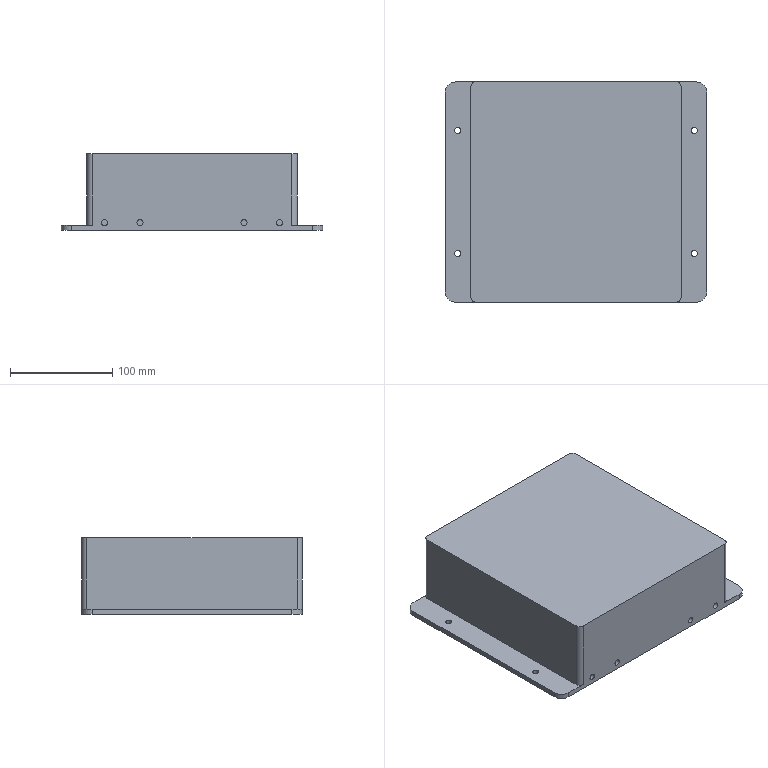NC program | NX | posted with a generic post | part box 255 x 215 x 75 mm
Lines 119 to 1998 of 11258:
(FLOOR_WALL_1_COPY_1 , TOOL : D16)
N224 T18 M6
N226 G54
N228 G17 G0 G90 X-0.676 Y-8. B0. C0. S9500 M3
N230 G43 Z30. H18
N232 Z1.5
N234 G94 G1 X3. Z1.307 F1000.
N236 Y8. Z0.469
N238 X-3. Z0.154
N240 Y-8. Z-0.684
N242 X3. Z-0.999
N244 Y8. F2500.
N246 X-3.
N248 Y-8.
N250 X3.
N252 Y-17.6
N254 X12.6
N256 Y17.6
N258 X-12.6
N260 Y-17.6
N262 X3.
N264 Y-27.2
N266 X22.2
N268 Y27.2
N270 X-22.2
N272 Y-27.2
N274 X3.
N276 Y-36.8
N278 X31.8
N280 Y36.8
N282 X-31.8
N284 Y-36.8
N286 X3.
N288 Y-46.4
N290 X41.4
N292 Y46.4
N294 X-41.4
N296 Y-46.4
N298 X3.
N300 Y-56.
N302 X51.
N304 Y56.
N306 X-51.
N308 Y-56.
N310 X3.
N312 Y-65.6
N314 X60.6
N316 Y65.6
N318 X-60.6
N320 Y-65.6
N322 X3.
N324 Y-75.2
N326 X70.2
N328 Y75.2
N330 X-70.2
N332 Y-75.2
N334 X3.
N336 Y-84.8
N338 X79.8
N340 Y84.8
N342 X-79.8
N344 Y-84.8
N346 X3.
N348 Y-94.4
N350 X89.4
N352 Y94.4
N354 X-89.4
N356 Y-94.4
N358 X3.
N360 Z0.501
N362 G0 X-0.676 Y-8.
N364 G1 X3. Z0.309 F1000.
N366 Y8. Z-0.53
N368 X-3. Z-0.844
N370 Y-8. Z-1.683
N372 X3. Z-1.997
N374 Y8. F2500.
N376 X-3.
N378 Y-8.
N380 X3.
N382 Y-17.6
N384 X12.6
N386 Y17.6
N388 X-12.6
N390 Y-17.6
N392 X3.
N394 Y-27.2
N396 X22.2
N398 Y27.2
N400 X-22.2
N402 Y-27.2
N404 X3.
N406 Y-36.8
N408 X31.8
N410 Y36.8
N412 X-31.8
N414 Y-36.8
N416 X3.
N418 Y-46.4
N420 X41.4
N422 Y46.4
N424 X-41.4
N426 Y-46.4
N428 X3.
N430 Y-56.
N432 X51.
N434 Y56.
N436 X-51.
N438 Y-56.
N440 X3.
N442 Y-65.6
N444 X60.6
N446 Y65.6
N448 X-60.6
N450 Y-65.6
N452 X3.
N454 Y-75.2
N456 X70.2
N458 Y75.2
N460 X-70.2
N462 Y-75.2
N464 X3.
N466 Y-84.8
N468 X79.8
N470 Y84.8
N472 X-79.8
N474 Y-84.8
N476 X3.
N478 Y-94.4
N480 X89.4
N482 Y94.4
N484 X-89.4
N486 Y-94.4
N488 X3.
N490 Z-0.497
N492 G0 X-0.676 Y-8.
N494 G1 X3. Z-0.69 F1000.
N496 Y8. Z-1.528
N498 X-3. Z-1.843
N500 Y-8. Z-2.681
N502 X3. Z-2.996
N504 Y8. F2500.
N506 X-3.
N508 Y-8.
N510 X3.
N512 Y-17.6
N514 X12.6
N516 Y17.6
N518 X-12.6
N520 Y-17.6
N522 X3.
N524 Y-27.2
N526 X22.2
N528 Y27.2
N530 X-22.2
N532 Y-27.2
N534 X3.
N536 Y-36.8
N538 X31.8
N540 Y36.8
N542 X-31.8
N544 Y-36.8
N546 X3.
N548 Y-46.4
N550 X41.4
N552 Y46.4
N554 X-41.4
N556 Y-46.4
N558 X3.
N560 Y-56.
N562 X51.
N564 Y56.
N566 X-51.
N568 Y-56.
N570 X3.
N572 Y-65.6
N574 X60.6
N576 Y65.6
N578 X-60.6
N580 Y-65.6
N582 X3.
N584 Y-75.2
N586 X70.2
N588 Y75.2
N590 X-70.2
N592 Y-75.2
N594 X3.
N596 Y-84.8
N598 X79.8
N600 Y84.8
N602 X-79.8
N604 Y-84.8
N606 X3.
N608 Y-94.4
N610 X89.4
N612 Y94.4
N614 X-89.4
N616 Y-94.4
N618 X3.
N620 Z-1.496
N622 G0 X-0.676 Y-8.
N624 G1 X3. Z-1.688 F1000.
N626 Y8. Z-2.527
N628 X-3. Z-2.841
N630 Y-8. Z-3.68
N632 X3. Z-3.994
N634 Y8. F2500.
N636 X-3.
N638 Y-8.
N640 X3.
N642 Y-17.6
N644 X12.6
N646 Y17.6
N648 X-12.6
N650 Y-17.6
N652 X3.
N654 Y-27.2
N656 X22.2
N658 Y27.2
N660 X-22.2
N662 Y-27.2
N664 X3.
N666 Y-36.8
N668 X31.8
N670 Y36.8
N672 X-31.8
N674 Y-36.8
N676 X3.
N678 Y-46.4
N680 X41.4
N682 Y46.4
N684 X-41.4
N686 Y-46.4
N688 X3.
N690 Y-56.
N692 X51.
N694 Y56.
N696 X-51.
N698 Y-56.
N700 X3.
N702 Y-65.6
N704 X60.6
N706 Y65.6
N708 X-60.6
N710 Y-65.6
N712 X3.
N714 Y-75.2
N716 X70.2
N718 Y75.2
N720 X-70.2
N722 Y-75.2
N724 X3.
N726 Y-84.8
N728 X79.8
N730 Y84.8
N732 X-79.8
N734 Y-84.8
N736 X3.
N738 Y-94.4
N740 X89.4
N742 Y94.4
N744 X-89.4
N746 Y-94.4
N748 X3.
N750 Z-2.494
N752 G0 X-0.676 Y-8.
N754 G1 X3. Z-2.687 F1000.
N756 Y8. Z-3.525
N758 X-3. Z-3.84
N760 Y-8. Z-4.678
N762 X3. Z-4.993
N764 Y8. F2500.
N766 X-3.
N768 Y-8.
N770 X3.
N772 Y-17.6
N774 X12.6
N776 Y17.6
N778 X-12.6
N780 Y-17.6
N782 X3.
N784 Y-27.2
N786 X22.2
N788 Y27.2
N790 X-22.2
N792 Y-27.2
N794 X3.
N796 Y-36.8
N798 X31.8
N800 Y36.8
N802 X-31.8
N804 Y-36.8
N806 X3.
N808 Y-46.4
N810 X41.4
N812 Y46.4
N814 X-41.4
N816 Y-46.4
N818 X3.
N820 Y-56.
N822 X51.
N824 Y56.
N826 X-51.
N828 Y-56.
N830 X3.
N832 Y-65.6
N834 X60.6
N836 Y65.6
N838 X-60.6
N840 Y-65.6
N842 X3.
N844 Y-75.2
N846 X70.2
N848 Y75.2
N850 X-70.2
N852 Y-75.2
N854 X3.
N856 Y-84.8
N858 X79.8
N860 Y84.8
N862 X-79.8
N864 Y-84.8
N866 X3.
N868 Y-94.4
N870 X89.4
N872 Y94.4
N874 X-89.4
N876 Y-94.4
N878 X3.
N880 Z-3.493
N882 G0 X-0.676 Y-8.
N884 G1 X3. Z-3.685 F1000.
N886 Y8. Z-4.524
N888 X-3. Z-4.838
N890 Y-8. Z-5.677
N892 X3. Z-5.991
N894 Y8. F2500.
N896 X-3.
N898 Y-8.
N900 X3.
N902 Y-17.6
N904 X12.6
N906 Y17.6
N908 X-12.6
N910 Y-17.6
N912 X3.
N914 Y-27.2
N916 X22.2
N918 Y27.2
N920 X-22.2
N922 Y-27.2
N924 X3.
N926 Y-36.8
N928 X31.8
N930 Y36.8
N932 X-31.8
N934 Y-36.8
N936 X3.
N938 Y-46.4
N940 X41.4
N942 Y46.4
N944 X-41.4
N946 Y-46.4
N948 X3.
N950 Y-56.
N952 X51.
N954 Y56.
N956 X-51.
N958 Y-56.
N960 X3.
N962 Y-65.6
N964 X60.6
N966 Y65.6
N968 X-60.6
N970 Y-65.6
N972 X3.
N974 Y-75.2
N976 X70.2
N978 Y75.2
N980 X-70.2
N982 Y-75.2
N984 X3.
N986 Y-84.8
N988 X79.8
N990 Y84.8
N992 X-79.8
N994 Y-84.8
N996 X3.
N998 Y-94.4
N1000 X89.4
N1002 Y94.4
N1004 X-89.4
N1006 Y-94.4
N1008 X3.
N1010 Z-4.491
N1012 G0 X-0.676 Y-8.
N1014 G1 X3. Z-4.684 F1000.
N1016 Y8. Z-5.523
N1018 X-3. Z-5.837
N1020 Y-8. Z-6.676
N1022 X3. Z-6.99
N1024 Y8. F2500.
N1026 X-3.
N1028 Y-8.
N1030 X3.
N1032 Y-17.6
N1034 X12.6
N1036 Y17.6
N1038 X-12.6
N1040 Y-17.6
N1042 X3.
N1044 Y-27.2
N1046 X22.2
N1048 Y27.2
N1050 X-22.2
N1052 Y-27.2
N1054 X3.
N1056 Y-36.8
N1058 X31.8
N1060 Y36.8
N1062 X-31.8
N1064 Y-36.8
N1066 X3.
N1068 Y-46.4
N1070 X41.4
N1072 Y46.4
N1074 X-41.4
N1076 Y-46.4
N1078 X3.
N1080 Y-56.
N1082 X51.
N1084 Y56.
N1086 X-51.
N1088 Y-56.
N1090 X3.
N1092 Y-65.6
N1094 X60.6
N1096 Y65.6
N1098 X-60.6
N1100 Y-65.6
N1102 X3.
N1104 Y-75.2
N1106 X70.2
N1108 Y75.2
N1110 X-70.2
N1112 Y-75.2
N1114 X3.
N1116 Y-84.8
N1118 X79.8
N1120 Y84.8
N1122 X-79.8
N1124 Y-84.8
N1126 X3.
N1128 Y-94.4
N1130 X89.4
N1132 Y94.4
N1134 X-89.4
N1136 Y-94.4
N1138 X3.
N1140 Z-5.49
N1142 G0 X-0.676 Y-8.
N1144 G1 X3. Z-5.683 F1000.
N1146 Y8. Z-6.521
N1148 X-3. Z-6.836
N1150 Y-8. Z-7.674
N1152 X3. Z-7.989
N1154 Y8. F2500.
N1156 X-3.
N1158 Y-8.
N1160 X3.
N1162 Y-17.6
N1164 X12.6
N1166 Y17.6
N1168 X-12.6
N1170 Y-17.6
N1172 X3.
N1174 Y-27.2
N1176 X22.2
N1178 Y27.2
N1180 X-22.2
N1182 Y-27.2
N1184 X3.
N1186 Y-36.8
N1188 X31.8
N1190 Y36.8
N1192 X-31.8
N1194 Y-36.8
N1196 X3.
N1198 Y-46.4
N1200 X41.4
N1202 Y46.4
N1204 X-41.4
N1206 Y-46.4
N1208 X3.
N1210 Y-56.
N1212 X51.
N1214 Y56.
N1216 X-51.
N1218 Y-56.
N1220 X3.
N1222 Y-65.6
N1224 X60.6
N1226 Y65.6
N1228 X-60.6
N1230 Y-65.6
N1232 X3.
N1234 Y-75.2
N1236 X70.2
N1238 Y75.2
N1240 X-70.2
N1242 Y-75.2
N1244 X3.
N1246 Y-84.8
N1248 X79.8
N1250 Y84.8
N1252 X-79.8
N1254 Y-84.8
N1256 X3.
N1258 Y-94.4
N1260 X89.4
N1262 Y94.4
N1264 X-89.4
N1266 Y-94.4
N1268 X3.
N1270 Z-6.489
N1272 G0 X-0.676 Y-8.
N1274 G1 X3. Z-6.681 F1000.
N1276 Y8. Z-7.52
N1278 X-3. Z-7.834
N1280 Y-8. Z-8.673
N1282 X3. Z-8.987
N1284 Y8. F2500.
N1286 X-3.
N1288 Y-8.
N1290 X3.
N1292 Y-17.6
N1294 X12.6
N1296 Y17.6
N1298 X-12.6
N1300 Y-17.6
N1302 X3.
N1304 Y-27.2
N1306 X22.2
N1308 Y27.2
N1310 X-22.2
N1312 Y-27.2
N1314 X3.
N1316 Y-36.8
N1318 X31.8
N1320 Y36.8
N1322 X-31.8
N1324 Y-36.8
N1326 X3.
N1328 Y-46.4
N1330 X41.4
N1332 Y46.4
N1334 X-41.4
N1336 Y-46.4
N1338 X3.
N1340 Y-56.
N1342 X51.
N1344 Y56.
N1346 X-51.
N1348 Y-56.
N1350 X3.
N1352 Y-65.6
N1354 X60.6
N1356 Y65.6
N1358 X-60.6
N1360 Y-65.6
N1362 X3.
N1364 Y-75.2
N1366 X70.2
N1368 Y75.2
N1370 X-70.2
N1372 Y-75.2
N1374 X3.
N1376 Y-84.8
N1378 X79.8
N1380 Y84.8
N1382 X-79.8
N1384 Y-84.8
N1386 X3.
N1388 Y-94.4
N1390 X89.4
N1392 Y94.4
N1394 X-89.4
N1396 Y-94.4
N1398 X3.
N1400 Z-7.487
N1402 G0 X-0.676 Y-8.
N1404 G1 X3. Z-7.68 F1000.
N1406 Y8. Z-8.518
N1408 X-3. Z-8.833
N1410 Y-8. Z-9.671
N1412 X3. Z-9.986
N1414 Y8. F2500.
N1416 X-3.
N1418 Y-8.
N1420 X3.
N1422 Y-17.6
N1424 X12.6
N1426 Y17.6
N1428 X-12.6
N1430 Y-17.6
N1432 X3.
N1434 Y-27.2
N1436 X22.2
N1438 Y27.2
N1440 X-22.2
N1442 Y-27.2
N1444 X3.
N1446 Y-36.8
N1448 X31.8
N1450 Y36.8
N1452 X-31.8
N1454 Y-36.8
N1456 X3.
N1458 Y-46.4
N1460 X41.4
N1462 Y46.4
N1464 X-41.4
N1466 Y-46.4
N1468 X3.
N1470 Y-56.
N1472 X51.
N1474 Y56.
N1476 X-51.
N1478 Y-56.
N1480 X3.
N1482 Y-65.6
N1484 X60.6
N1486 Y65.6
N1488 X-60.6
N1490 Y-65.6
N1492 X3.
N1494 Y-75.2
N1496 X70.2
N1498 Y75.2
N1500 X-70.2
N1502 Y-75.2
N1504 X3.
N1506 Y-84.8
N1508 X79.8
N1510 Y84.8
N1512 X-79.8
N1514 Y-84.8
N1516 X3.
N1518 Y-94.4
N1520 X89.4
N1522 Y94.4
N1524 X-89.4
N1526 Y-94.4
N1528 X3.
N1530 Z-8.486
N1532 G0 X-0.676 Y-8.
N1534 G1 X3. Z-8.678 F1000.
N1536 Y8. Z-9.517
N1538 X-3. Z-9.831
N1540 Y-8. Z-10.67
N1542 X3. Z-10.984
N1544 Y8. F2500.
N1546 X-3.
N1548 Y-8.
N1550 X3.
N1552 Y-17.6
N1554 X12.6
N1556 Y17.6
N1558 X-12.6
N1560 Y-17.6
N1562 X3.
N1564 Y-27.2
N1566 X22.2
N1568 Y27.2
N1570 X-22.2
N1572 Y-27.2
N1574 X3.
N1576 Y-36.8
N1578 X31.8
N1580 Y36.8
N1582 X-31.8
N1584 Y-36.8
N1586 X3.
N1588 Y-46.4
N1590 X41.4
N1592 Y46.4
N1594 X-41.4
N1596 Y-46.4
N1598 X3.
N1600 Y-56.
N1602 X51.
N1604 Y56.
N1606 X-51.
N1608 Y-56.
N1610 X3.
N1612 Y-65.6
N1614 X60.6
N1616 Y65.6
N1618 X-60.6
N1620 Y-65.6
N1622 X3.
N1624 Y-75.2
N1626 X70.2
N1628 Y75.2
N1630 X-70.2
N1632 Y-75.2
N1634 X3.
N1636 Y-84.8
N1638 X79.8
N1640 Y84.8
N1642 X-79.8
N1644 Y-84.8
N1646 X3.
N1648 Y-94.4
N1650 X89.4
N1652 Y94.4
N1654 X-89.4
N1656 Y-94.4
N1658 X3.
N1660 Z-9.484
N1662 G0 X-0.676 Y-8.
N1664 G1 X3. Z-9.677 F1000.
N1666 Y8. Z-10.515
N1668 X-3. Z-10.83
N1670 Y-8. Z-11.668
N1672 X3. Z-11.983
N1674 Y8. F2500.
N1676 X-3.
N1678 Y-8.
N1680 X3.
N1682 Y-17.6
N1684 X12.6
N1686 Y17.6
N1688 X-12.6
N1690 Y-17.6
N1692 X3.
N1694 Y-27.2
N1696 X22.2
N1698 Y27.2
N1700 X-22.2
N1702 Y-27.2
N1704 X3.
N1706 Y-36.8
N1708 X31.8
N1710 Y36.8
N1712 X-31.8
N1714 Y-36.8
N1716 X3.
N1718 Y-46.4
N1720 X41.4
N1722 Y46.4
N1724 X-41.4
N1726 Y-46.4
N1728 X3.
N1730 Y-56.
N1732 X51.
N1734 Y56.
N1736 X-51.
N1738 Y-56.
N1740 X3.
N1742 Y-65.6
N1744 X60.6
N1746 Y65.6
N1748 X-60.6
N1750 Y-65.6
N1752 X3.
N1754 Y-75.2
N1756 X70.2
N1758 Y75.2
N1760 X-70.2
N1762 Y-75.2
N1764 X3.
N1766 Y-84.8
N1768 X79.8
N1770 Y84.8
N1772 X-79.8
N1774 Y-84.8
N1776 X3.
N1778 Y-94.4
N1780 X89.4
N1782 Y94.4
N1784 X-89.4
N1786 Y-94.4
N1788 X3.
N1790 Z-10.483
N1792 G0 X-0.676 Y-8.
N1794 G1 X3. Z-10.675 F1000.
N1796 Y8. Z-11.514
N1798 X-3. Z-11.828
N1800 Y-8. Z-12.667
N1802 X3. Z-12.981
N1804 Y8. F2500.
N1806 X-3.
N1808 Y-8.
N1810 X3.
N1812 Y-17.6
N1814 X12.6
N1816 Y17.6
N1818 X-12.6
N1820 Y-17.6
N1822 X3.
N1824 Y-27.2
N1826 X22.2
N1828 Y27.2
N1830 X-22.2
N1832 Y-27.2
N1834 X3.
N1836 Y-36.8
N1838 X31.8
N1840 Y36.8
N1842 X-31.8
N1844 Y-36.8
N1846 X3.
N1848 Y-46.4
N1850 X41.4
N1852 Y46.4
N1854 X-41.4
N1856 Y-46.4
N1858 X3.
N1860 Y-56.
N1862 X51.
N1864 Y56.
N1866 X-51.
N1868 Y-56.
N1870 X3.
N1872 Y-65.6
N1874 X60.6
N1876 Y65.6
N1878 X-60.6
N1880 Y-65.6
N1882 X3.
N1884 Y-75.2
N1886 X70.2
N1888 Y75.2
N1890 X-70.2
N1892 Y-75.2
N1894 X3.
N1896 Y-84.8
N1898 X79.8
N1900 Y84.8
N1902 X-79.8
N1904 Y-84.8
N1906 X3.
N1908 Y-94.4
N1910 X89.4
N1912 Y94.4
N1914 X-89.4
N1916 Y-94.4
N1918 X3.
N1920 Z-11.481
N1922 G0 X-0.676 Y-8.
N1924 G1 X3. Z-11.674 F1000.
N1926 Y8. Z-12.513
N1928 X-3. Z-12.827
N1930 Y-8. Z-13.666
N1932 X3. Z-13.98
N1934 Y8. F2500.
N1936 X-3.
N1938 Y-8.
N1940 X3.
N1942 Y-17.6
N1944 X12.6
N1946 Y17.6
N1948 X-12.6
N1950 Y-17.6
N1952 X3.
N1954 Y-27.2
N1956 X22.2
N1958 Y27.2
N1960 X-22.2
N1962 Y-27.2
N1964 X3.
N1966 Y-36.8
N1968 X31.8
N1970 Y36.8
N1972 X-31.8
N1974 Y-36.8
N1976 X3.
N1978 Y-46.4
N1980 X41.4
N1982 Y46.4
N1984 X-41.4
N1986 Y-46.4
N1988 X3.
N1990 Y-56.
N1992 X51.
N1994 Y56.
N1996 X-51.
N1998 Y-56.
N2000 X3.
N2002 Y-65.6
N2004 X60.6
N2006 Y65.6
N2008 X-60.6
N2010 Y-65.6
N2012 X3.
N2014 Y-75.2
N2016 X70.2
N2018 Y75.2
N2020 X-70.2
N2022 Y-75.2
N2024 X3.
N2026 Y-84.8
N2028 X79.8
N2030 Y84.8
N2032 X-79.8
N2034 Y-84.8
N2036 X3.
N2038 Y-94.4
N2040 X89.4
N2042 Y94.4
N2044 X-89.4
N2046 Y-94.4
N2048 X3.
N2050 Z-12.48
N2052 G0 X-0.676 Y-8.
N2054 G1 X3. Z-12.673 F1000.
N2056 Y8. Z-13.511
N2058 X-3. Z-13.826
N2060 Y-8. Z-14.664
N2062 X3. Z-14.979
N2064 Y8. F2500.
N2066 X-3.
N2068 Y-8.
N2070 X3.
N2072 Y-17.6
N2074 X12.6
N2076 Y17.6
N2078 X-12.6
N2080 Y-17.6
N2082 X3.
N2084 Y-27.2
N2086 X22.2
N2088 Y27.2
N2090 X-22.2
N2092 Y-27.2
N2094 X3.
N2096 Y-36.8
N2098 X31.8
N2100 Y36.8
N2102 X-31.8
N2104 Y-36.8
N2106 X3.
N2108 Y-46.4
N2110 X41.4
N2112 Y46.4
N2114 X-41.4
N2116 Y-46.4
N2118 X3.
N2120 Y-56.
N2122 X51.
N2124 Y56.
N2126 X-51.
N2128 Y-56.
N2130 X3.
N2132 Y-65.6
N2134 X60.6
N2136 Y65.6
N2138 X-60.6
N2140 Y-65.6
N2142 X3.
N2144 Y-75.2
N2146 X70.2
N2148 Y75.2
N2150 X-70.2
N2152 Y-75.2
N2154 X3.
N2156 Y-84.8
N2158 X79.8
N2160 Y84.8
N2162 X-79.8
N2164 Y-84.8
N2166 X3.
N2168 Y-94.4
N2170 X89.4
N2172 Y94.4
N2174 X-89.4
N2176 Y-94.4
N2178 X3.
N2180 Z-13.479
N2182 G0 X-0.676 Y-8.
N2184 G1 X3. Z-13.671 F1000.
N2186 Y8. Z-14.51
N2188 X-3. Z-14.824
N2190 Y-8. Z-15.663
N2192 X3. Z-15.977
N2194 Y8. F2500.
N2196 X-3.
N2198 Y-8.
N2200 X3.
N2202 Y-17.6
N2204 X12.6
N2206 Y17.6
N2208 X-12.6
N2210 Y-17.6
N2212 X3.
N2214 Y-27.2
N2216 X22.2
N2218 Y27.2
N2220 X-22.2
N2222 Y-27.2
N2224 X3.
N2226 Y-36.8
N2228 X31.8
N2230 Y36.8
N2232 X-31.8
N2234 Y-36.8
N2236 X3.
N2238 Y-46.4
N2240 X41.4
N2242 Y46.4
N2244 X-41.4
N2246 Y-46.4
N2248 X3.
N2250 Y-56.
N2252 X51.
N2254 Y56.
N2256 X-51.
N2258 Y-56.
N2260 X3.
N2262 Y-65.6
N2264 X60.6
N2266 Y65.6
N2268 X-60.6
N2270 Y-65.6
N2272 X3.
N2274 Y-75.2
N2276 X70.2
N2278 Y75.2
N2280 X-70.2
N2282 Y-75.2
N2284 X3.
N2286 Y-84.8
N2288 X79.8
N2290 Y84.8
N2292 X-79.8
N2294 Y-84.8
N2296 X3.
N2298 Y-94.4
N2300 X89.4
N2302 Y94.4
N2304 X-89.4
N2306 Y-94.4
N2308 X3.
N2310 Z-14.477
N2312 G0 X-0.676 Y-8.
N2314 G1 X3. Z-14.67 F1000.
N2316 Y8. Z-15.508
N2318 X-3. Z-15.823
N2320 Y-8. Z-16.661
N2322 X3. Z-16.976
N2324 Y8. F2500.
N2326 X-3.
N2328 Y-8.
N2330 X3.
N2332 Y-17.6
N2334 X12.6
N2336 Y17.6
N2338 X-12.6
N2340 Y-17.6
N2342 X3.
N2344 Y-27.2
N2346 X22.2
N2348 Y27.2
N2350 X-22.2
N2352 Y-27.2
N2354 X3.
N2356 Y-36.8
N2358 X31.8
N2360 Y36.8
N2362 X-31.8
N2364 Y-36.8
N2366 X3.
N2368 Y-46.4
N2370 X41.4
N2372 Y46.4
N2374 X-41.4
N2376 Y-46.4
N2378 X3.
N2380 Y-56.
N2382 X51.
N2384 Y56.
N2386 X-51.
N2388 Y-56.
N2390 X3.
N2392 Y-65.6
N2394 X60.6
N2396 Y65.6
N2398 X-60.6
N2400 Y-65.6
N2402 X3.
N2404 Y-75.2
N2406 X70.2
N2408 Y75.2
N2410 X-70.2
N2412 Y-75.2
N2414 X3.
N2416 Y-84.8
N2418 X79.8
N2420 Y84.8
N2422 X-79.8
N2424 Y-84.8
N2426 X3.
N2428 Y-94.4
N2430 X89.4
N2432 Y94.4
N2434 X-89.4
N2436 Y-94.4
N2438 X3.
N2440 Z-15.476
N2442 G0 X-0.676 Y-8.
N2444 G1 X3. Z-15.668 F1000.
N2446 Y8. Z-16.507
N2448 X-3. Z-16.821
N2450 Y-8. Z-17.66
N2452 X3. Z-17.974
N2454 Y8. F2500.
N2456 X-3.
N2458 Y-8.
N2460 X3.
N2462 Y-17.6
N2464 X12.6
N2466 Y17.6
N2468 X-12.6
N2470 Y-17.6
N2472 X3.
N2474 Y-27.2
N2476 X22.2
N2478 Y27.2
N2480 X-22.2
N2482 Y-27.2
N2484 X3.
N2486 Y-36.8
N2488 X31.8
N2490 Y36.8
N2492 X-31.8
N2494 Y-36.8
N2496 X3.
N2498 Y-46.4
N2500 X41.4
N2502 Y46.4
N2504 X-41.4
N2506 Y-46.4
N2508 X3.
N2510 Y-56.
N2512 X51.
N2514 Y56.
N2516 X-51.
N2518 Y-56.
N2520 X3.
N2522 Y-65.6
N2524 X60.6
N2526 Y65.6
N2528 X-60.6
N2530 Y-65.6
N2532 X3.
N2534 Y-75.2
N2536 X70.2
N2538 Y75.2
N2540 X-70.2
N2542 Y-75.2
N2544 X3.
N2546 Y-84.8
N2548 X79.8
N2550 Y84.8
N2552 X-79.8
N2554 Y-84.8
N2556 X3.
N2558 Y-94.4
N2560 X89.4
N2562 Y94.4
N2564 X-89.4
N2566 Y-94.4
N2568 X3.
N2570 Z-16.474
N2572 G0 X-0.676 Y-8.
N2574 G1 X3. Z-16.667 F1000.
N2576 Y8. Z-17.505
N2578 X-3. Z-17.82
N2580 Y-8. Z-18.658
N2582 X3. Z-18.973
N2584 Y8. F2500.
N2586 X-3.
N2588 Y-8.
N2590 X3.
N2592 Y-17.6
N2594 X12.6
N2596 Y17.6
N2598 X-12.6
N2600 Y-17.6
N2602 X3.
N2604 Y-27.2
N2606 X22.2
N2608 Y27.2
N2610 X-22.2
N2612 Y-27.2
N2614 X3.
N2616 Y-36.8
N2618 X31.8
N2620 Y36.8
N2622 X-31.8
N2624 Y-36.8
N2626 X3.
N2628 Y-46.4
N2630 X41.4
N2632 Y46.4
N2634 X-41.4
N2636 Y-46.4
N2638 X3.
N2640 Y-56.
N2642 X51.
N2644 Y56.
N2646 X-51.
N2648 Y-56.
N2650 X3.
N2652 Y-65.6
N2654 X60.6
N2656 Y65.6
N2658 X-60.6
N2660 Y-65.6
N2662 X3.
N2664 Y-75.2
N2666 X70.2
N2668 Y75.2
N2670 X-70.2
N2672 Y-75.2
N2674 X3.
N2676 Y-84.8
N2678 X79.8
N2680 Y84.8
N2682 X-79.8
N2684 Y-84.8
N2686 X3.
N2688 Y-94.4
N2690 X89.4
N2692 Y94.4
N2694 X-89.4
N2696 Y-94.4
N2698 X3.
N2700 Z-17.473
N2702 G0 X-0.676 Y-8.
N2704 G1 X3. Z-17.665 F1000.
N2706 Y8. Z-18.504
N2708 X-3. Z-18.818
N2710 Y-8. Z-19.657
N2712 X3. Z-19.971
N2714 Y8. F2500.
N2716 X-3.
N2718 Y-8.
N2720 X3.
N2722 Y-17.6
N2724 X12.6
N2726 Y17.6
N2728 X-12.6
N2730 Y-17.6
N2732 X3.
N2734 Y-27.2
N2736 X22.2
N2738 Y27.2
N2740 X-22.2
N2742 Y-27.2
N2744 X3.
N2746 Y-36.8
N2748 X31.8
N2750 Y36.8
N2752 X-31.8
N2754 Y-36.8
N2756 X3.
N2758 Y-46.4
N2760 X41.4
N2762 Y46.4
N2764 X-41.4
N2766 Y-46.4
N2768 X3.
N2770 Y-56.
N2772 X51.
N2774 Y56.
N2776 X-51.
N2778 Y-56.
N2780 X3.
N2782 Y-65.6
N2784 X60.6
N2786 Y65.6
N2788 X-60.6
N2790 Y-65.6
N2792 X3.
N2794 Y-75.2
N2796 X70.2
N2798 Y75.2
N2800 X-70.2
N2802 Y-75.2
N2804 X3.
N2806 Y-84.8
N2808 X79.8
N2810 Y84.8
N2812 X-79.8
N2814 Y-84.8
N2816 X3.
N2818 Y-94.4
N2820 X89.4
N2822 Y94.4
N2824 X-89.4
N2826 Y-94.4
N2828 X3.
N2830 Z-18.471
N2832 G0 X-0.676 Y-8.
N2834 G1 X3. Z-18.664 F1000.
N2836 Y8. Z-19.503
N2838 X-3. Z-19.817
N2840 Y-8. Z-20.656
N2842 X3. Z-20.97
N2844 Y8. F2500.
N2846 X-3.
N2848 Y-8.
N2850 X3.
N2852 Y-17.6
N2854 X12.6
N2856 Y17.6
N2858 X-12.6
N2860 Y-17.6
N2862 X3.
N2864 Y-27.2
N2866 X22.2
N2868 Y27.2
N2870 X-22.2
N2872 Y-27.2
N2874 X3.
N2876 Y-36.8
N2878 X31.8
N2880 Y36.8
N2882 X-31.8
N2884 Y-36.8
N2886 X3.
N2888 Y-46.4
N2890 X41.4
N2892 Y46.4
N2894 X-41.4
N2896 Y-46.4
N2898 X3.
N2900 Y-56.
N2902 X51.
N2904 Y56.
N2906 X-51.
N2908 Y-56.
N2910 X3.
N2912 Y-65.6
N2914 X60.6
N2916 Y65.6
N2918 X-60.6
N2920 Y-65.6
N2922 X3.
N2924 Y-75.2
N2926 X70.2
N2928 Y75.2
N2930 X-70.2
N2932 Y-75.2
N2934 X3.
N2936 Y-84.8
N2938 X79.8
N2940 Y84.8
N2942 X-79.8
N2944 Y-84.8
N2946 X3.
N2948 Y-94.4
N2950 X89.4
N2952 Y94.4
N2954 X-89.4
N2956 Y-94.4
N2958 X3.
N2960 Z-19.47
N2962 G0 X-0.676 Y-8.
N2964 G1 X3. Z-19.663 F1000.
N2966 Y8. Z-20.501
N2968 X-3. Z-20.816
N2970 Y-8. Z-21.654
N2972 X3. Z-21.969
N2974 Y8. F2500.
N2976 X-3.
N2978 Y-8.
N2980 X3.
N2982 Y-17.6
N2984 X12.6
N2986 Y17.6
N2988 X-12.6
N2990 Y-17.6
N2992 X3.
N2994 Y-27.2
N2996 X22.2
N2998 Y27.2
N3000 X-22.2
N3002 Y-27.2
N3004 X3.
N3006 Y-36.8
N3008 X31.8
N3010 Y36.8
N3012 X-31.8
N3014 Y-36.8
N3016 X3.
N3018 Y-46.4
N3020 X41.4
N3022 Y46.4
N3024 X-41.4
N3026 Y-46.4
N3028 X3.
N3030 Y-56.
N3032 X51.
N3034 Y56.
N3036 X-51.
N3038 Y-56.
N3040 X3.
N3042 Y-65.6
N3044 X60.6
N3046 Y65.6
N3048 X-60.6
N3050 Y-65.6
N3052 X3.
N3054 Y-75.2
N3056 X70.2
N3058 Y75.2
N3060 X-70.2
N3062 Y-75.2
N3064 X3.
N3066 Y-84.8
N3068 X79.8
N3070 Y84.8
N3072 X-79.8
N3074 Y-84.8
N3076 X3.
N3078 Y-94.4
N3080 X89.4
N3082 Y94.4
N3084 X-89.4
N3086 Y-94.4
N3088 X3.
N3090 Z-20.469
N3092 G0 X-0.676 Y-8.
N3094 G1 X3. Z-20.661 F1000.
N3096 Y8. Z-21.5
N3098 X-3. Z-21.814
N3100 Y-8. Z-22.653
N3102 X3. Z-22.967
N3104 Y8. F2500.
N3106 X-3.
N3108 Y-8.
N3110 X3.
N3112 Y-17.6
N3114 X12.6
N3116 Y17.6
N3118 X-12.6
N3120 Y-17.6
N3122 X3.
N3124 Y-27.2
N3126 X22.2
N3128 Y27.2
N3130 X-22.2
N3132 Y-27.2
N3134 X3.
N3136 Y-36.8
N3138 X31.8
N3140 Y36.8
N3142 X-31.8
N3144 Y-36.8
N3146 X3.
N3148 Y-46.4
N3150 X41.4
N3152 Y46.4
N3154 X-41.4
N3156 Y-46.4
N3158 X3.
N3160 Y-56.
N3162 X51.
N3164 Y56.
N3166 X-51.
N3168 Y-56.
N3170 X3.
N3172 Y-65.6
N3174 X60.6
N3176 Y65.6
N3178 X-60.6
N3180 Y-65.6
N3182 X3.
N3184 Y-75.2
N3186 X70.2
N3188 Y75.2
N3190 X-70.2
N3192 Y-75.2
N3194 X3.
N3196 Y-84.8
N3198 X79.8
N3200 Y84.8
N3202 X-79.8
N3204 Y-84.8
N3206 X3.
N3208 Y-94.4
N3210 X89.4
N3212 Y94.4
N3214 X-89.4
N3216 Y-94.4
N3218 X3.
N3220 Z-21.467
N3222 G0 X-0.676 Y-8.
N3224 G1 X3. Z-21.66 F1000.
N3226 Y8. Z-22.498
N3228 X-3. Z-22.813
N3230 Y-8. Z-23.651
N3232 X3. Z-23.966
N3234 Y8. F2500.
N3236 X-3.
N3238 Y-8.
N3240 X3.
N3242 Y-17.6
N3244 X12.6
N3246 Y17.6
N3248 X-12.6
N3250 Y-17.6
N3252 X3.
N3254 Y-27.2
N3256 X22.2
N3258 Y27.2
N3260 X-22.2
N3262 Y-27.2
N3264 X3.
N3266 Y-36.8
N3268 X31.8
N3270 Y36.8
N3272 X-31.8
N3274 Y-36.8
N3276 X3.
N3278 Y-46.4
N3280 X41.4
N3282 Y46.4
N3284 X-41.4
N3286 Y-46.4
N3288 X3.
N3290 Y-56.
N3292 X51.
N3294 Y56.
N3296 X-51.
N3298 Y-56.
N3300 X3.
N3302 Y-65.6
N3304 X60.6
N3306 Y65.6
N3308 X-60.6
N3310 Y-65.6
N3312 X3.
N3314 Y-75.2
N3316 X70.2
N3318 Y75.2
N3320 X-70.2
N3322 Y-75.2
N3324 X3.
N3326 Y-84.8
N3328 X79.8
N3330 Y84.8
N3332 X-79.8
N3334 Y-84.8
N3336 X3.
N3338 Y-94.4
N3340 X89.4
N3342 Y94.4
N3344 X-89.4
N3346 Y-94.4
N3348 X3.
N3350 Z-22.466
N3352 G0 X-0.676 Y-8.
N3354 G1 X3. Z-22.658 F1000.
N3356 Y8. Z-23.497
N3358 X-3. Z-23.811
N3360 Y-8. Z-24.65
N3362 X3. Z-24.964
N3364 Y8. F2500.
N3366 X-3.
N3368 Y-8.
N3370 X3.
N3372 Y-17.6
N3374 X12.6
N3376 Y17.6
N3378 X-12.6
N3380 Y-17.6
N3382 X3.
N3384 Y-27.2
N3386 X22.2
N3388 Y27.2
N3390 X-22.2
N3392 Y-27.2
N3394 X3.
N3396 Y-36.8
N3398 X31.8
N3400 Y36.8
N3402 X-31.8
N3404 Y-36.8
N3406 X3.
N3408 Y-46.4
N3410 X41.4
N3412 Y46.4
N3414 X-41.4
N3416 Y-46.4
N3418 X3.
N3420 Y-56.
N3422 X51.
N3424 Y56.
N3426 X-51.
N3428 Y-56.
N3430 X3.
N3432 Y-65.6
N3434 X60.6
N3436 Y65.6
N3438 X-60.6
N3440 Y-65.6
N3442 X3.
N3444 Y-75.2
N3446 X70.2
N3448 Y75.2
N3450 X-70.2
N3452 Y-75.2
N3454 X3.
N3456 Y-84.8
N3458 X79.8
N3460 Y84.8
N3462 X-79.8
N3464 Y-84.8
N3466 X3.
N3468 Y-94.4
N3470 X89.4
N3472 Y94.4
N3474 X-89.4
N3476 Y-94.4
N3478 X3.
N3480 Z-23.464
N3482 G0 X-0.676 Y-8.
N3484 G1 X3. Z-23.657 F1000.
N3486 Y8. Z-24.495
N3488 X-3. Z-24.81
N3490 Y-8. Z-25.648
N3492 X3. Z-25.963
N3494 Y8. F2500.
N3496 X-3.
N3498 Y-8.
N3500 X3.
N3502 Y-17.6
N3504 X12.6
N3506 Y17.6
N3508 X-12.6
N3510 Y-17.6
N3512 X3.
N3514 Y-27.2
N3516 X22.2
N3518 Y27.2
N3520 X-22.2
N3522 Y-27.2
N3524 X3.
N3526 Y-36.8
N3528 X31.8
N3530 Y36.8
N3532 X-31.8
N3534 Y-36.8
N3536 X3.
N3538 Y-46.4
N3540 X41.4
N3542 Y46.4
N3544 X-41.4
N3546 Y-46.4
N3548 X3.
N3550 Y-56.
N3552 X51.
N3554 Y56.
N3556 X-51.
N3558 Y-56.
N3560 X3.
N3562 Y-65.6
N3564 X60.6
N3566 Y65.6
N3568 X-60.6
N3570 Y-65.6
N3572 X3.
N3574 Y-75.2
N3576 X70.2
N3578 Y75.2
N3580 X-70.2
N3582 Y-75.2
N3584 X3.
N3586 Y-84.8
N3588 X79.8
N3590 Y84.8
N3592 X-79.8
N3594 Y-84.8
N3596 X3.
N3598 Y-94.4
N3600 X89.4
N3602 Y94.4
N3604 X-89.4
N3606 Y-94.4
N3608 X3.
N3610 Z-24.463
N3612 G0 X-0.676 Y-8.
N3614 G1 X3. Z-24.655 F1000.
N3616 Y8. Z-25.494
N3618 X-3. Z-25.808
N3620 Y-8. Z-26.647
N3622 X3. Z-26.961
N3624 Y8. F2500.
N3626 X-3.
N3628 Y-8.
N3630 X3.
N3632 Y-17.6
N3634 X12.6
N3636 Y17.6
N3638 X-12.6
N3640 Y-17.6
N3642 X3.
N3644 Y-27.2
N3646 X22.2
N3648 Y27.2
N3650 X-22.2
N3652 Y-27.2
N3654 X3.
N3656 Y-36.8
N3658 X31.8
N3660 Y36.8
N3662 X-31.8
N3664 Y-36.8
N3666 X3.
N3668 Y-46.4
N3670 X41.4
N3672 Y46.4
N3674 X-41.4
N3676 Y-46.4
N3678 X3.
N3680 Y-56.
N3682 X51.
N3684 Y56.
N3686 X-51.
N3688 Y-56.
N3690 X3.
N3692 Y-65.6
N3694 X60.6
N3696 Y65.6
N3698 X-60.6
N3700 Y-65.6
N3702 X3.
N3704 Y-75.2
N3706 X70.2
N3708 Y75.2
N3710 X-70.2
N3712 Y-75.2
N3714 X3.
N3716 Y-84.8
N3718 X79.8
N3720 Y84.8
N3722 X-79.8
N3724 Y-84.8
N3726 X3.
N3728 Y-94.4
N3730 X89.4
N3732 Y94.4
N3734 X-89.4
N3736 Y-94.4
N3738 X3.
N3740 Z-25.461
N3742 G0 X-0.676 Y-8.
N3744 G1 X3. Z-25.654 F1000.
N3746 Y8. Z-26.493
N3748 X-3. Z-26.807
N3750 Y-8. Z-27.646
N3752 X3. Z-27.96
N3754 Y8. F2500.
N3756 X-3.
N3758 Y-8.
N3760 X3.
N3762 Y-17.6
N3764 X12.6
N3766 Y17.6
N3768 X-12.6
N3770 Y-17.6
N3772 X3.
N3774 Y-27.2
N3776 X22.2
N3778 Y27.2
N3780 X-22.2
N3782 Y-27.2
N3784 X3.
N3786 Y-36.8
N3788 X31.8
N3790 Y36.8
N3792 X-31.8
N3794 Y-36.8
N3796 X3.
N3798 Y-46.4
N3800 X41.4
N3802 Y46.4
N3804 X-41.4
N3806 Y-46.4
N3808 X3.
N3810 Y-56.
N3812 X51.
N3814 Y56.
N3816 X-51.
N3818 Y-56.
N3820 X3.
N3822 Y-65.6
N3824 X60.6
N3826 Y65.6
N3828 X-60.6
N3830 Y-65.6
N3832 X3.
N3834 Y-75.2
N3836 X70.2
N3838 Y75.2
N3840 X-70.2
N3842 Y-75.2
N3844 X3.
N3846 Y-84.8
N3848 X79.8
N3850 Y84.8
N3852 X-79.8
N3854 Y-84.8
N3856 X3.
N3858 Y-94.4
N3860 X89.4
N3862 Y94.4
N3864 X-89.4
N3866 Y-94.4
N3868 X3.
N3870 Z-26.46
N3872 G0 X-0.676 Y-8.
N3874 G1 X3. Z-26.653 F1000.
N3876 Y8. Z-27.491
N3878 X-3. Z-27.806
N3880 Y-8. Z-28.644
N3882 X3. Z-28.959
N3884 Y8. F2500.
N3886 X-3.
N3888 Y-8.
N3890 X3.
N3892 Y-17.6
N3894 X12.6
N3896 Y17.6
N3898 X-12.6
N3900 Y-17.6
N3902 X3.
N3904 Y-27.2
N3906 X22.2
N3908 Y27.2
N3910 X-22.2
N3912 Y-27.2
N3914 X3.
N3916 Y-36.8
N3918 X31.8
N3920 Y36.8
N3922 X-31.8
N3924 Y-36.8
N3926 X3.
N3928 Y-46.4
N3930 X41.4
N3932 Y46.4
N3934 X-41.4
N3936 Y-46.4
N3938 X3.
N3940 Y-56.
N3942 X51.
N3944 Y56.
N3946 X-51.
N3948 Y-56.
N3950 X3.
N3952 Y-65.6
N3954 X60.6
N3956 Y65.6
N3958 X-60.6
N3960 Y-65.6
N3962 X3.
N3964 Y-75.2
N3966 X70.2
N3968 Y75.2
N3970 X-70.2
N3972 Y-75.2
N3974 X3.
N3976 Y-84.8